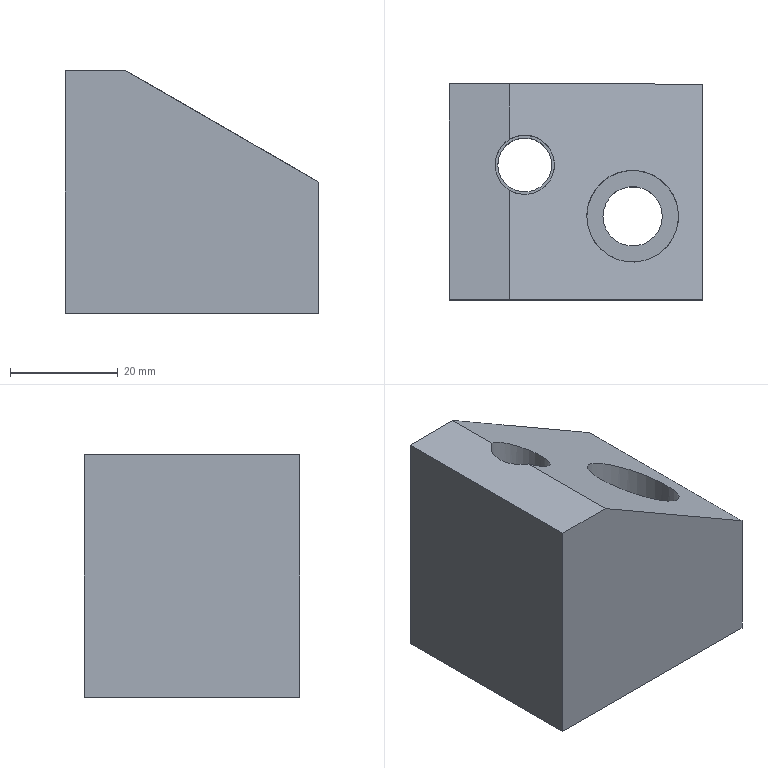Part | STEP file | lll_id4630_x_t | 1 solid | 13 faces | box 47 x 40 x 45 mm | volume 60683 mm3 | plane 9 | cylinder 4 | commonest cylinder face diameters 11 x2 10 x1 17 x1
STEP:
#1=CARTESIAN_POINT('',(3900.715,20.,0.));
#2=VERTEX_POINT('',#1);
#3=CARTESIAN_POINT('',(3936.5,20.,-20.66));
#4=VERTEX_POINT('',#3);
#5=CARTESIAN_POINT('',(3917.262,20.,-9.553));
#6=DIRECTION('',(0.866,0.,-0.5));
#7=VECTOR('',#6,1.);
#8=LINE('',#5,#7);
#9=EDGE_CURVE('',#2,#4,#8,.T.);
#10=ORIENTED_EDGE('',*,*,#9,.F.);
#11=CARTESIAN_POINT('',(3900.715,9.743,0.));
#12=VERTEX_POINT('',#11);
#13=CARTESIAN_POINT('',(3900.715,-7.,0.));
#14=DIRECTION('',(0.,1.,0.));
#15=VECTOR('',#14,1.);
#16=LINE('',#13,#15);
#17=EDGE_CURVE('',#12,#2,#16,.T.);
#18=ORIENTED_EDGE('',*,*,#17,.F.);
#19=CARTESIAN_POINT('',(3900.715,0.2571,0.));
#20=VERTEX_POINT('',#19);
#21=CARTESIAN_POINT('',(3903.5,5.,-1.608));
#22=DIRECTION('',(0.5,0.,0.866));
#23=DIRECTION('',(0.866,0.,-0.5));
#24=AXIS2_PLACEMENT_3D('',#21,#22,#23);
#25=ELLIPSE('',#24,6.351,5.5);
#26=EDGE_CURVE('',#20,#12,#25,.T.);
#27=ORIENTED_EDGE('',*,*,#26,.F.);
#28=CARTESIAN_POINT('',(3900.715,-20.,0.));
#29=VERTEX_POINT('',#28);
#30=CARTESIAN_POINT('',(3900.715,-7.,0.));
#31=DIRECTION('',(0.,1.,0.));
#32=VECTOR('',#31,1.);
#33=LINE('',#30,#32);
#34=EDGE_CURVE('',#29,#20,#33,.T.);
#35=ORIENTED_EDGE('',*,*,#34,.F.);
#36=CARTESIAN_POINT('',(3936.5,-20.,-20.66));
#37=VERTEX_POINT('',#36);
#38=CARTESIAN_POINT('',(3917.262,-20.,-9.553));
#39=DIRECTION('',(-0.866,0.,0.5));
#40=VECTOR('',#39,1.);
#41=LINE('',#38,#40);
#42=EDGE_CURVE('',#37,#29,#41,.T.);
#43=ORIENTED_EDGE('',*,*,#42,.F.);
#44=CARTESIAN_POINT('',(3936.5,-7.,-20.66));
#45=DIRECTION('',(0.,-1.,0.));
#46=VECTOR('',#45,1.);
#47=LINE('',#44,#46);
#48=EDGE_CURVE('',#4,#37,#47,.T.);
#49=ORIENTED_EDGE('',*,*,#48,.F.);
#50=EDGE_LOOP('',(#10,#18,#27,#35,#43,#49));
#51=FACE_BOUND('',#50,.T.);
#52=CARTESIAN_POINT('',(3915.,-4.5,-8.247));
#53=VERTEX_POINT('',#52);
#54=CARTESIAN_POINT('',(3923.5,-4.5,-13.155));
#55=DIRECTION('',(0.5,0.,0.866));
#56=DIRECTION('',(-0.866,0.,0.5));
#57=AXIS2_PLACEMENT_3D('',#54,#55,#56);
#58=ELLIPSE('',#57,9.815,8.5);
#59=EDGE_CURVE('',#53,#53,#58,.T.);
#60=ORIENTED_EDGE('',*,*,#59,.F.);
#61=EDGE_LOOP('',(#60));
#62=FACE_BOUND('',#61,.T.);
#63=CARTESIAN_POINT('',(3911.215,-36.5,-6.062));
#64=DIRECTION('',(-0.5,0.,-0.866));
#65=DIRECTION('',(-0.866,0.,0.5));
#66=AXIS2_PLACEMENT_3D('',#63,#64,#65);
#67=PLANE('',#66);
#68=ADVANCED_FACE('',(#51,#62),#67,.F.);
#69=CARTESIAN_POINT('',(3898.5,5.,-15.));
#70=VERTEX_POINT('',#69);
#71=CARTESIAN_POINT('',(3903.5,5.,-15.));
#72=DIRECTION('',(0.,0.,1.));
#73=DIRECTION('',(-1.,0.,0.));
#74=AXIS2_PLACEMENT_3D('',#71,#72,#73);
#75=CIRCLE('',#74,5.);
#76=EDGE_CURVE('',#70,#70,#75,.T.);
#77=ORIENTED_EDGE('',*,*,#76,.T.);
#78=EDGE_LOOP('',(#77));
#79=FACE_BOUND('',#78,.T.);
#80=CARTESIAN_POINT('',(3898.5,5.,-45.));
#81=VERTEX_POINT('',#80);
#82=CARTESIAN_POINT('',(3903.5,5.,-45.));
#83=DIRECTION('',(0.,0.,1.));
#84=DIRECTION('',(-1.,0.,0.));
#85=AXIS2_PLACEMENT_3D('',#82,#83,#84);
#86=CIRCLE('',#85,5.);
#87=EDGE_CURVE('',#81,#81,#86,.T.);
#88=ORIENTED_EDGE('',*,*,#87,.F.);
#89=EDGE_LOOP('',(#88));
#90=FACE_BOUND('',#89,.T.);
#91=CARTESIAN_POINT('',(3903.5,5.,-20.));
#92=DIRECTION('',(0.,0.,-1.));
#93=DIRECTION('',(-1.,0.,0.));
#94=AXIS2_PLACEMENT_3D('',#91,#92,#93);
#95=CYLINDRICAL_SURFACE('',#94,5.);
#96=ADVANCED_FACE('',(#79,#90),#95,.F.);
#97=CARTESIAN_POINT('',(3898.,5.,-15.));
#98=VERTEX_POINT('',#97);
#99=CARTESIAN_POINT('',(3903.5,5.,-15.));
#100=DIRECTION('',(0.,0.,1.));
#101=DIRECTION('',(-1.,0.,0.));
#102=AXIS2_PLACEMENT_3D('',#99,#100,#101);
#103=CIRCLE('',#102,5.5);
#104=EDGE_CURVE('',#98,#98,#103,.T.);
#105=ORIENTED_EDGE('',*,*,#104,.T.);
#106=EDGE_LOOP('',(#105));
#107=FACE_BOUND('',#106,.T.);
#108=ORIENTED_EDGE('',*,*,#76,.F.);
#109=EDGE_LOOP('',(#108));
#110=FACE_BOUND('',#109,.T.);
#111=CARTESIAN_POINT('',(3903.5,5.,-15.));
#112=DIRECTION('',(0.,0.,-1.));
#113=DIRECTION('',(-1.,0.,0.));
#114=AXIS2_PLACEMENT_3D('',#111,#112,#113);
#115=PLANE('',#114);
#116=ADVANCED_FACE('',(#107,#110),#115,.F.);
#117=CARTESIAN_POINT('',(3889.5,20.,-45.));
#118=VERTEX_POINT('',#117);
#119=CARTESIAN_POINT('',(3889.5,-20.,-45.));
#120=VERTEX_POINT('',#119);
#121=CARTESIAN_POINT('',(3889.5,-7.,-45.));
#122=DIRECTION('',(0.,-1.,0.));
#123=VECTOR('',#122,1.);
#124=LINE('',#121,#123);
#125=EDGE_CURVE('',#118,#120,#124,.T.);
#126=ORIENTED_EDGE('',*,*,#125,.T.);
#127=CARTESIAN_POINT('',(3889.5,-20.,0.));
#128=VERTEX_POINT('',#127);
#129=CARTESIAN_POINT('',(3889.5,-20.,-65.));
#130=DIRECTION('',(0.,0.,-1.));
#131=VECTOR('',#130,1.);
#132=LINE('',#129,#131);
#133=EDGE_CURVE('',#128,#120,#132,.T.);
#134=ORIENTED_EDGE('',*,*,#133,.F.);
#135=CARTESIAN_POINT('',(3889.5,20.,0.));
#136=VERTEX_POINT('',#135);
#137=CARTESIAN_POINT('',(3889.5,-7.,0.));
#138=DIRECTION('',(0.,1.,0.));
#139=VECTOR('',#138,1.);
#140=LINE('',#137,#139);
#141=EDGE_CURVE('',#128,#136,#140,.T.);
#142=ORIENTED_EDGE('',*,*,#141,.T.);
#143=CARTESIAN_POINT('',(3889.5,20.,-65.));
#144=DIRECTION('',(0.,0.,-1.));
#145=VECTOR('',#144,1.);
#146=LINE('',#143,#145);
#147=EDGE_CURVE('',#136,#118,#146,.T.);
#148=ORIENTED_EDGE('',*,*,#147,.T.);
#149=EDGE_LOOP('',(#126,#134,#142,#148));
#150=FACE_OUTER_BOUND('',#149,.T.);
#151=CARTESIAN_POINT('',(3889.5,-7.,-65.));
#152=DIRECTION('',(-1.,0.,0.));
#153=DIRECTION('',(0.,0.,-1.));
#154=AXIS2_PLACEMENT_3D('',#151,#152,#153);
#155=PLANE('',#154);
#156=ADVANCED_FACE('',(#150),#155,.T.);
#157=CARTESIAN_POINT('',(3885.25,20.,0.));
#158=DIRECTION('',(1.,0.,0.));
#159=VECTOR('',#158,1.);
#160=LINE('',#157,#159);
#161=EDGE_CURVE('',#136,#2,#160,.T.);
#162=ORIENTED_EDGE('',*,*,#161,.T.);
#163=ORIENTED_EDGE('',*,*,#9,.T.);
#164=CARTESIAN_POINT('',(3936.5,20.,-45.));
#165=VERTEX_POINT('',#164);
#166=CARTESIAN_POINT('',(3936.5,20.,-65.));
#167=DIRECTION('',(0.,0.,-1.));
#168=VECTOR('',#167,1.);
#169=LINE('',#166,#168);
#170=EDGE_CURVE('',#4,#165,#169,.T.);
#171=ORIENTED_EDGE('',*,*,#170,.T.);
#172=CARTESIAN_POINT('',(3885.25,20.,-45.));
#173=DIRECTION('',(-1.,0.,0.));
#174=VECTOR('',#173,1.);
#175=LINE('',#172,#174);
#176=EDGE_CURVE('',#165,#118,#175,.T.);
#177=ORIENTED_EDGE('',*,*,#176,.T.);
#178=ORIENTED_EDGE('',*,*,#147,.F.);
#179=EDGE_LOOP('',(#162,#163,#171,#177,#178));
#180=FACE_OUTER_BOUND('',#179,.T.);
#181=CARTESIAN_POINT('',(3885.25,20.,-65.));
#182=DIRECTION('',(0.,1.,0.));
#183=DIRECTION('',(0.,0.,-1.));
#184=AXIS2_PLACEMENT_3D('',#181,#182,#183);
#185=PLANE('',#184);
#186=ADVANCED_FACE('',(#180),#185,.T.);
#187=ORIENTED_EDGE('',*,*,#170,.F.);
#188=ORIENTED_EDGE('',*,*,#48,.T.);
#189=CARTESIAN_POINT('',(3936.5,-20.,-45.));
#190=VERTEX_POINT('',#189);
#191=CARTESIAN_POINT('',(3936.5,-20.,-65.));
#192=DIRECTION('',(0.,0.,-1.));
#193=VECTOR('',#192,1.);
#194=LINE('',#191,#193);
#195=EDGE_CURVE('',#37,#190,#194,.T.);
#196=ORIENTED_EDGE('',*,*,#195,.T.);
#197=CARTESIAN_POINT('',(3936.5,-7.,-45.));
#198=DIRECTION('',(0.,1.,0.));
#199=VECTOR('',#198,1.);
#200=LINE('',#197,#199);
#201=EDGE_CURVE('',#190,#165,#200,.T.);
#202=ORIENTED_EDGE('',*,*,#201,.T.);
#203=EDGE_LOOP('',(#187,#188,#196,#202));
#204=FACE_OUTER_BOUND('',#203,.T.);
#205=CARTESIAN_POINT('',(3936.5,-7.,-65.));
#206=DIRECTION('',(1.,0.,0.));
#207=DIRECTION('',(0.,0.,1.));
#208=AXIS2_PLACEMENT_3D('',#205,#206,#207);
#209=PLANE('',#208);
#210=ADVANCED_FACE('',(#204),#209,.T.);
#211=ORIENTED_EDGE('',*,*,#195,.F.);
#212=ORIENTED_EDGE('',*,*,#42,.T.);
#213=CARTESIAN_POINT('',(3885.25,-20.,0.));
#214=DIRECTION('',(-1.,0.,0.));
#215=VECTOR('',#214,1.);
#216=LINE('',#213,#215);
#217=EDGE_CURVE('',#29,#128,#216,.T.);
#218=ORIENTED_EDGE('',*,*,#217,.T.);
#219=ORIENTED_EDGE('',*,*,#133,.T.);
#220=CARTESIAN_POINT('',(3885.25,-20.,-45.));
#221=DIRECTION('',(1.,0.,0.));
#222=VECTOR('',#221,1.);
#223=LINE('',#220,#222);
#224=EDGE_CURVE('',#120,#190,#223,.T.);
#225=ORIENTED_EDGE('',*,*,#224,.T.);
#226=EDGE_LOOP('',(#211,#212,#218,#219,#225));
#227=FACE_OUTER_BOUND('',#226,.T.);
#228=CARTESIAN_POINT('',(3885.25,-20.,-65.));
#229=DIRECTION('',(0.,-1.,0.));
#230=DIRECTION('',(0.,0.,1.));
#231=AXIS2_PLACEMENT_3D('',#228,#229,#230);
#232=PLANE('',#231);
#233=ADVANCED_FACE('',(#227),#232,.T.);
#234=CARTESIAN_POINT('',(3918.,-4.5,-45.));
#235=VERTEX_POINT('',#234);
#236=CARTESIAN_POINT('',(3923.5,-4.5,-45.));
#237=DIRECTION('',(0.,0.,-1.));
#238=DIRECTION('',(-1.,0.,0.));
#239=AXIS2_PLACEMENT_3D('',#236,#237,#238);
#240=CIRCLE('',#239,5.5);
#241=EDGE_CURVE('',#235,#235,#240,.T.);
#242=ORIENTED_EDGE('',*,*,#241,.F.);
#243=EDGE_LOOP('',(#242));
#244=FACE_BOUND('',#243,.T.);
#245=ORIENTED_EDGE('',*,*,#87,.T.);
#246=EDGE_LOOP('',(#245));
#247=FACE_BOUND('',#246,.T.);
#248=ORIENTED_EDGE('',*,*,#224,.F.);
#249=ORIENTED_EDGE('',*,*,#125,.F.);
#250=ORIENTED_EDGE('',*,*,#176,.F.);
#251=ORIENTED_EDGE('',*,*,#201,.F.);
#252=EDGE_LOOP('',(#248,#249,#250,#251));
#253=FACE_BOUND('',#252,.T.);
#254=CARTESIAN_POINT('',(3885.25,-7.,-45.));
#255=DIRECTION('',(0.,0.,-1.));
#256=DIRECTION('',(1.,0.,0.));
#257=AXIS2_PLACEMENT_3D('',#254,#255,#256);
#258=PLANE('',#257);
#259=ADVANCED_FACE('',(#244,#247,#253),#258,.T.);
#260=ORIENTED_EDGE('',*,*,#104,.F.);
#261=EDGE_LOOP('',(#260));
#262=FACE_BOUND('',#261,.T.);
#263=ORIENTED_EDGE('',*,*,#26,.T.);
#264=CARTESIAN_POINT('',(3903.5,5.,0.));
#265=DIRECTION('',(0.,0.,1.));
#266=DIRECTION('',(1.,0.,0.));
#267=AXIS2_PLACEMENT_3D('',#264,#265,#266);
#268=CIRCLE('',#267,5.5);
#269=EDGE_CURVE('',#12,#20,#268,.T.);
#270=ORIENTED_EDGE('',*,*,#269,.T.);
#271=EDGE_LOOP('',(#263,#270));
#272=FACE_BOUND('',#271,.T.);
#273=CARTESIAN_POINT('',(3903.5,5.,0.));
#274=DIRECTION('',(0.,0.,-1.));
#275=DIRECTION('',(-1.,0.,0.));
#276=AXIS2_PLACEMENT_3D('',#273,#274,#275);
#277=CYLINDRICAL_SURFACE('',#276,5.5);
#278=ADVANCED_FACE('',(#262,#272),#277,.F.);
#279=ORIENTED_EDGE('',*,*,#269,.F.);
#280=ORIENTED_EDGE('',*,*,#17,.T.);
#281=ORIENTED_EDGE('',*,*,#161,.F.);
#282=ORIENTED_EDGE('',*,*,#141,.F.);
#283=ORIENTED_EDGE('',*,*,#217,.F.);
#284=ORIENTED_EDGE('',*,*,#34,.T.);
#285=EDGE_LOOP('',(#279,#280,#281,#282,#283,#284));
#286=FACE_OUTER_BOUND('',#285,.T.);
#287=CARTESIAN_POINT('',(3885.25,-7.,0.));
#288=DIRECTION('',(0.,0.,1.));
#289=DIRECTION('',(-1.,0.,0.));
#290=AXIS2_PLACEMENT_3D('',#287,#288,#289);
#291=PLANE('',#290);
#292=ADVANCED_FACE('',(#286),#291,.T.);
#293=ORIENTED_EDGE('',*,*,#59,.T.);
#294=EDGE_LOOP('',(#293));
#295=FACE_BOUND('',#294,.T.);
#296=CARTESIAN_POINT('',(3915.,-4.5,-32.));
#297=VERTEX_POINT('',#296);
#298=CARTESIAN_POINT('',(3923.5,-4.5,-32.));
#299=DIRECTION('',(0.,0.,1.));
#300=DIRECTION('',(-1.,0.,0.));
#301=AXIS2_PLACEMENT_3D('',#298,#299,#300);
#302=CIRCLE('',#301,8.5);
#303=EDGE_CURVE('',#297,#297,#302,.T.);
#304=ORIENTED_EDGE('',*,*,#303,.F.);
#305=EDGE_LOOP('',(#304));
#306=FACE_BOUND('',#305,.T.);
#307=CARTESIAN_POINT('',(3923.5,-4.5,-20.));
#308=DIRECTION('',(0.,0.,1.));
#309=DIRECTION('',(-1.,0.,0.));
#310=AXIS2_PLACEMENT_3D('',#307,#308,#309);
#311=CYLINDRICAL_SURFACE('',#310,8.5);
#312=ADVANCED_FACE('',(#295,#306),#311,.F.);
#313=CARTESIAN_POINT('',(3918.,-4.5,-32.));
#314=VERTEX_POINT('',#313);
#315=CARTESIAN_POINT('',(3923.5,-4.5,-32.));
#316=DIRECTION('',(0.,0.,-1.));
#317=DIRECTION('',(-1.,0.,0.));
#318=AXIS2_PLACEMENT_3D('',#315,#316,#317);
#319=CIRCLE('',#318,5.5);
#320=EDGE_CURVE('',#314,#314,#319,.T.);
#321=ORIENTED_EDGE('',*,*,#320,.T.);
#322=EDGE_LOOP('',(#321));
#323=FACE_BOUND('',#322,.T.);
#324=ORIENTED_EDGE('',*,*,#303,.T.);
#325=EDGE_LOOP('',(#324));
#326=FACE_BOUND('',#325,.T.);
#327=CARTESIAN_POINT('',(3923.5,-4.5,-32.));
#328=DIRECTION('',(0.,0.,-1.));
#329=DIRECTION('',(1.,0.,0.));
#330=AXIS2_PLACEMENT_3D('',#327,#328,#329);
#331=PLANE('',#330);
#332=ADVANCED_FACE('',(#323,#326),#331,.F.);
#333=ORIENTED_EDGE('',*,*,#320,.F.);
#334=EDGE_LOOP('',(#333));
#335=FACE_BOUND('',#334,.T.);
#336=ORIENTED_EDGE('',*,*,#241,.T.);
#337=EDGE_LOOP('',(#336));
#338=FACE_BOUND('',#337,.T.);
#339=CARTESIAN_POINT('',(3923.5,-4.5,-20.));
#340=DIRECTION('',(0.,0.,-1.));
#341=DIRECTION('',(1.,0.,0.));
#342=AXIS2_PLACEMENT_3D('',#339,#340,#341);
#343=CYLINDRICAL_SURFACE('',#342,5.5);
#344=ADVANCED_FACE('',(#335,#338),#343,.F.);
#345=CLOSED_SHELL('',(#68,#96,#116,#156,#186,#210,#233,#259,#278,#292,#312,#332,#344));
#346=MANIFOLD_SOLID_BREP('',#345);
#347=(LENGTH_UNIT()NAMED_UNIT(*)SI_UNIT(.MILLI.,.METRE.));
#348=UNCERTAINTY_MEASURE_WITH_UNIT(LENGTH_MEASURE(0.00002),#347,'','');
#349=(NAMED_UNIT(*)PLANE_ANGLE_UNIT()SI_UNIT($,.RADIAN.));
#350=PLANE_ANGLE_MEASURE_WITH_UNIT(PLANE_ANGLE_MEASURE(0.01745),#349);
#351=DIMENSIONAL_EXPONENTS(0.,0.,0.,0.,0.,0.,0.);
#352=(CONVERSION_BASED_UNIT('DEGREE',#350)NAMED_UNIT(#351)PLANE_ANGLE_UNIT());
#353=(NAMED_UNIT(*)SI_UNIT($,.STERADIAN.)SOLID_ANGLE_UNIT());
#354=(GEOMETRIC_REPRESENTATION_CONTEXT(3)GLOBAL_UNCERTAINTY_ASSIGNED_CONTEXT((#348))GLOBAL_UNIT_ASSIGNED_CONTEXT((#347,#352,#353))REPRESENTATION_CONTEXT('',''));
#355=ADVANCED_BREP_SHAPE_REPRESENTATION('',(#346),#354);